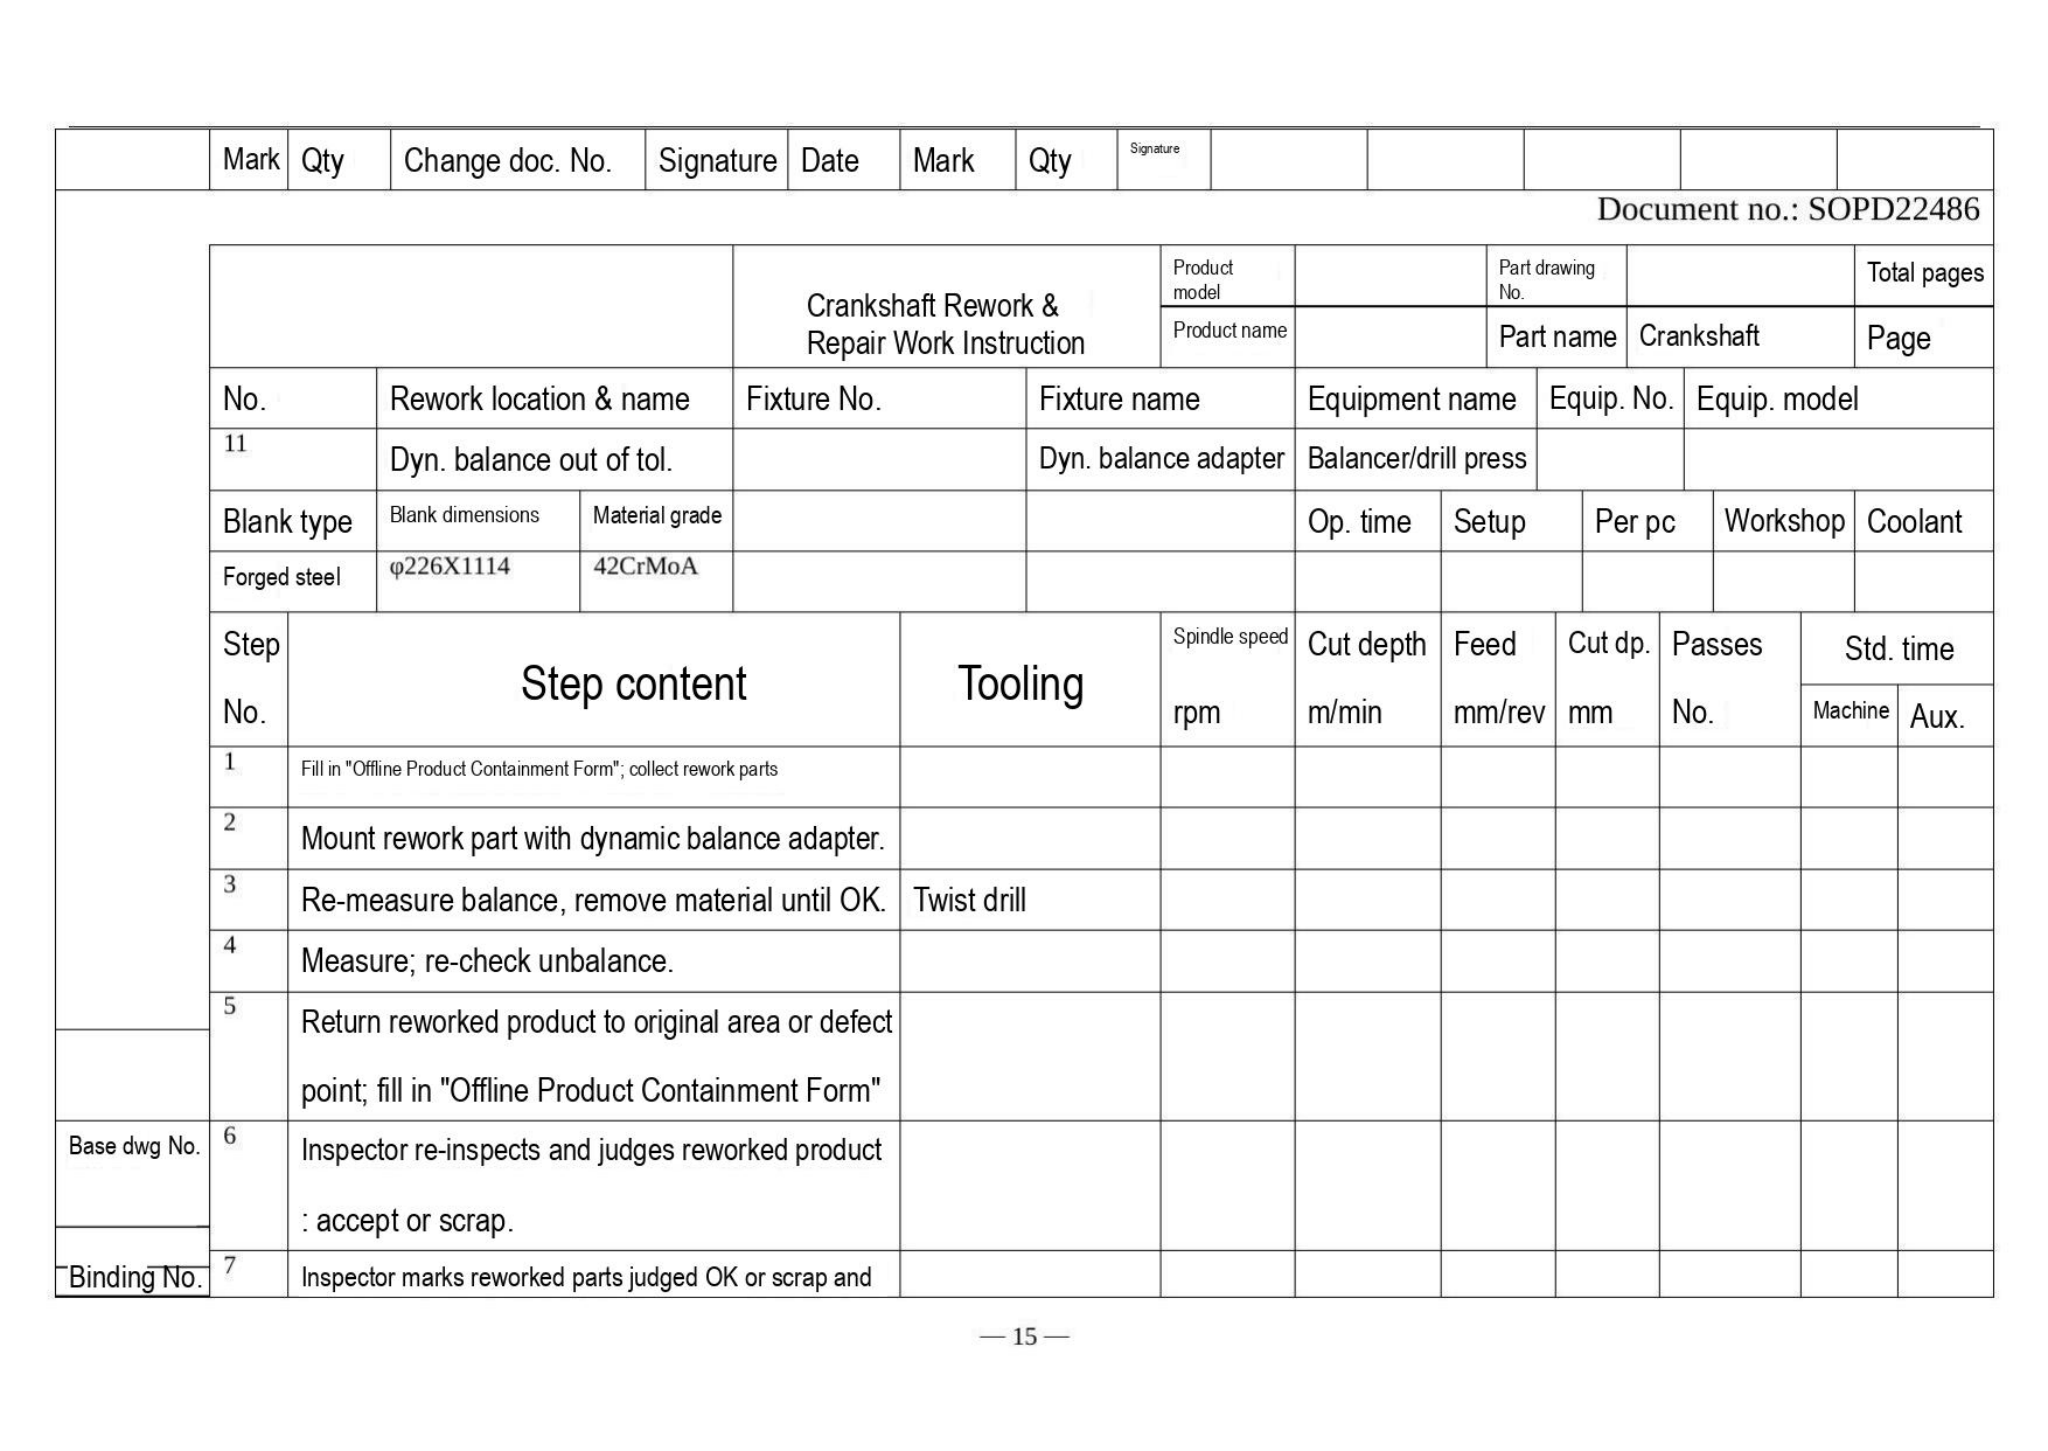| Mark | Qty | Change doc. No. | Signature | Date | Mark | Qty | Signature |
|---|---|---|---|---|---|---|---|

Document no.: SOPD22486

| | Crankshaft Rework & Repair Work Instruction | Product model | | Part drawing No. | | Total pages |
|---|---|---|---|---|---|---|
| | | Product name | | Part name | Crankshaft | Page |

| No. | Rework location & name | Fixture No. | Fixture name | Equipment name | Equip. No. | Equip. model |
|---|---|---|---|---|---|---|
| 11 | Dyn. balance out of tol. | | Dyn. balance adapter | Balancer/drill press | | |

| Blank type | Blank dimensions | Material grade | | | Op. time | Setup | Per pc | Workshop | Coolant |
|---|---|---|---|---|---|---|---|---|---|
| Forged steel | φ226X1114 | 42CrMoA | | | | | | | |

| Step No. | Step content | Tooling | Spindle speed rpm | Cut depth m/min | Feed mm/rev | Cut dp. mm | Passes No. | Std. time Machine | Std. time Aux. |
|---|---|---|---|---|---|---|---|---|---|
| 1 | Fill in "Offline Product Containment Form"; collect rework parts | | | | | | | | |
| 2 | Mount rework part with dynamic balance adapter. | | | | | | | | |
| 3 | Re-measure balance, remove material until OK. | Twist drill | | | | | | | |
| 4 | Measure; re-check unbalance. | | | | | | | | |
| 5 | Return reworked product to original area or defect point; fill in "Offline Product Containment Form" | | | | | | | | |
| 6 | Inspector re-inspects and judges reworked product : accept or scrap. | | | | | | | | |
| 7 | Inspector marks reworked parts judged OK or scrap and | | | | | | | | |

Base dwg No.

Binding No.

— 15 —
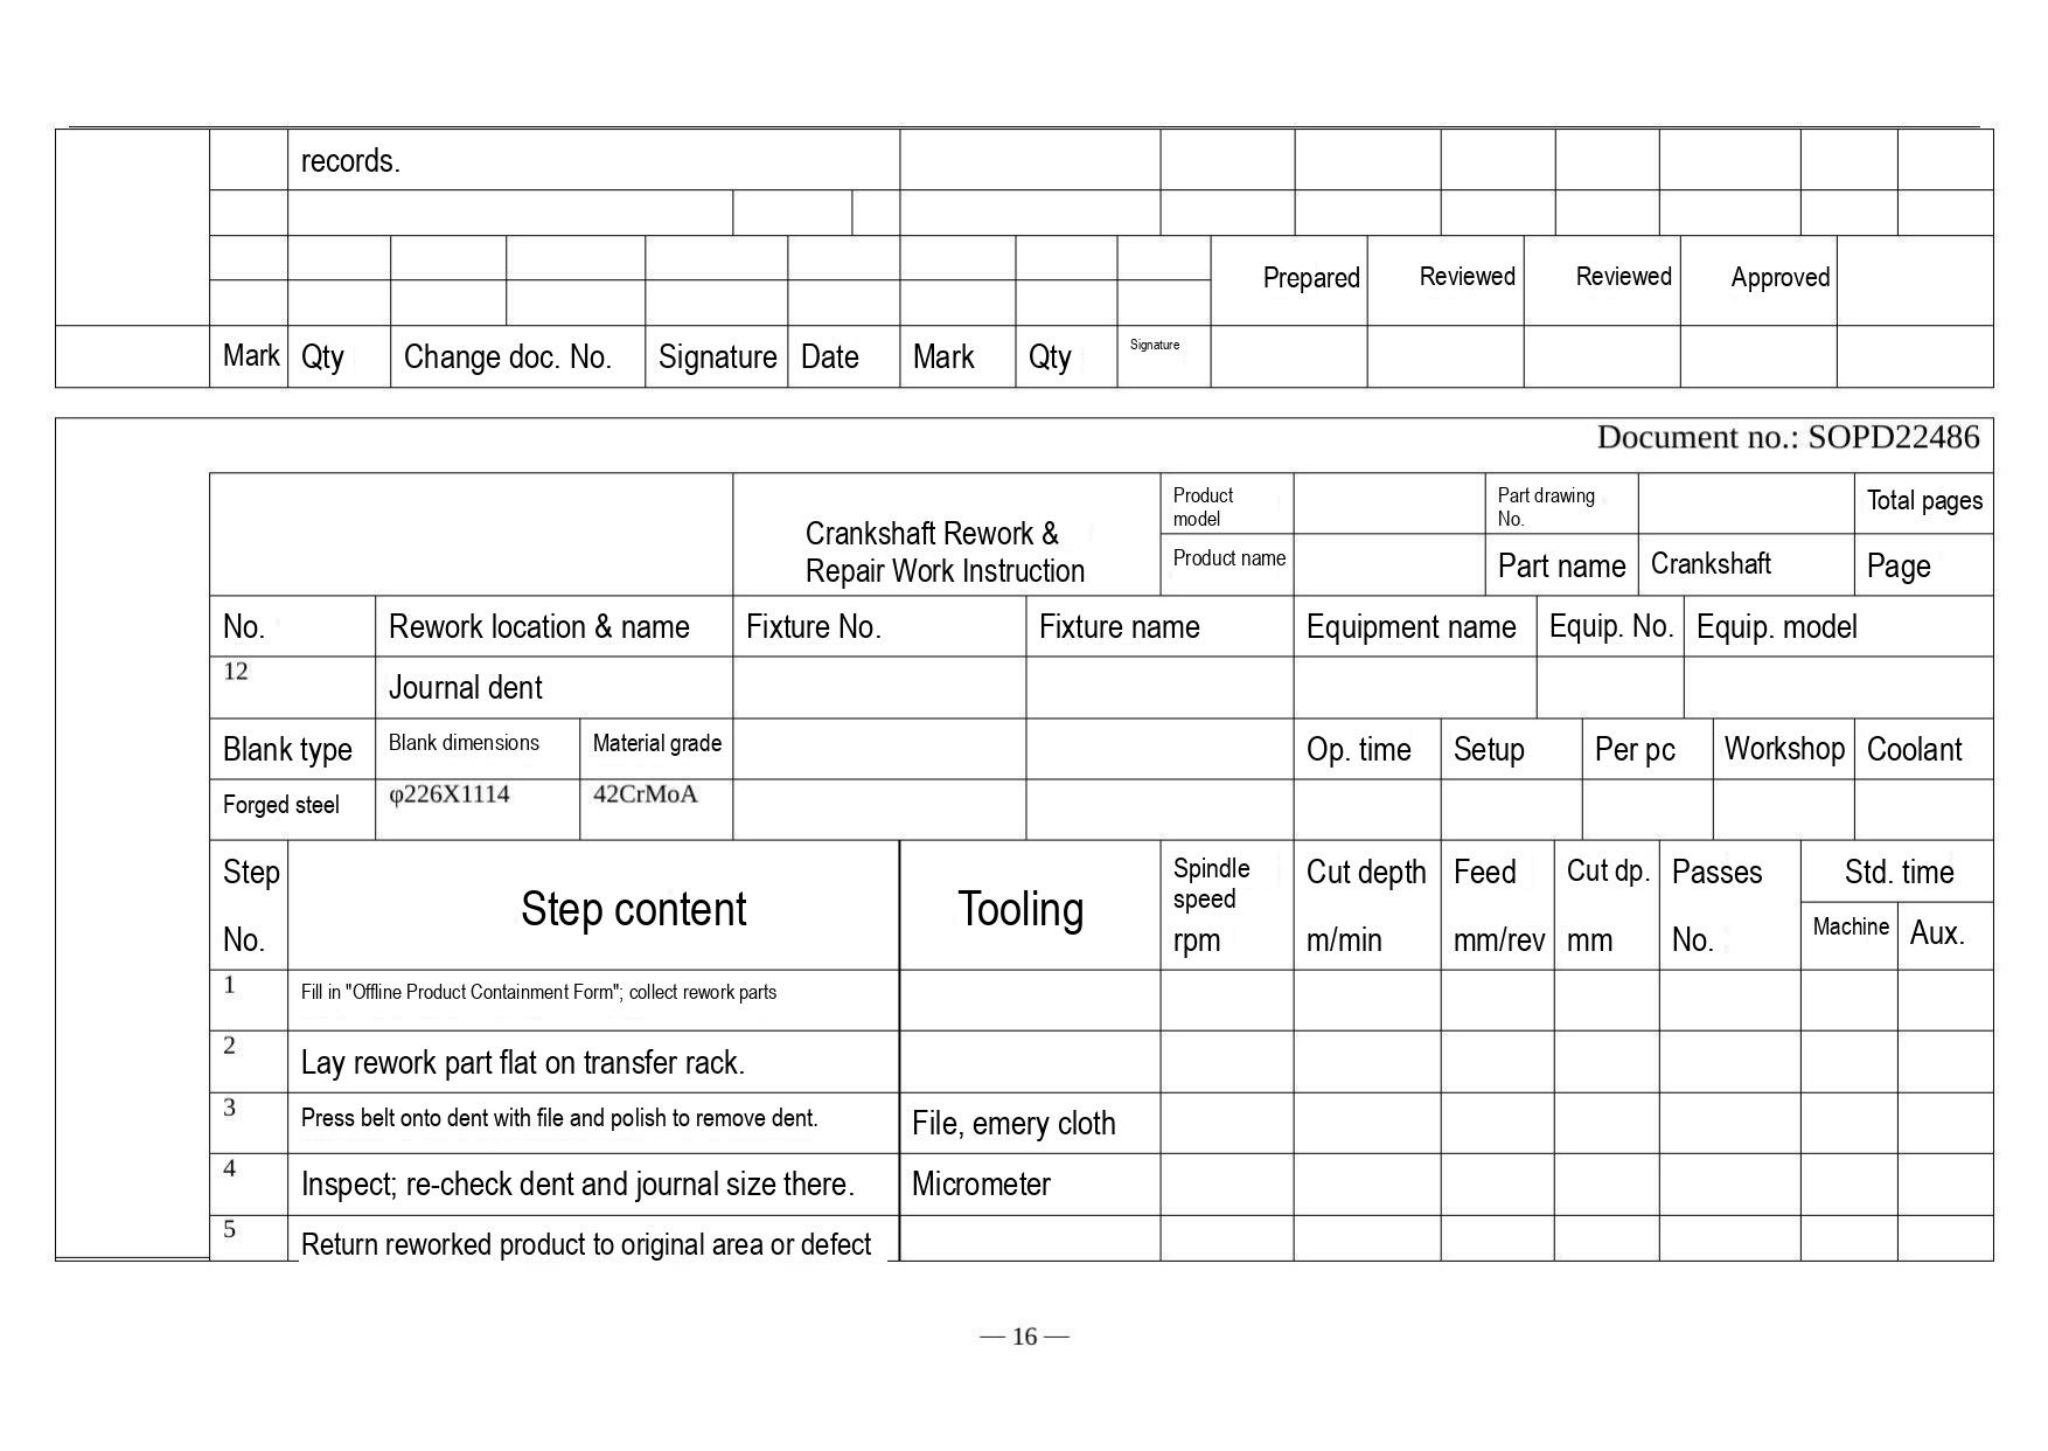| | | | | | | | | | | | | | |
|---|---|---|---|---|---|---|---|---|---|---|---|---|---|
| | records. | | | | | | | | | | | | |
| | | | | | | | | | | | | | |
| | | | | | | | | | Prepared | Reviewed | Reviewed | Approved | |
| Mark | Qty | Change doc. No. | Signature | Date | Mark | Qty | Signature | | | | | | |

Document no.: SOPD22486

| | Crankshaft Rework & Repair Work Instruction | Product model | | Part drawing No. | | Total pages |
|---|---|---|---|---|---|---|
| | | Product name | | Part name | Crankshaft | Page |

| No. | Rework location & name | Fixture No. | Fixture name | Equipment name | Equip. No. | Equip. model |
|---|---|---|---|---|---|---|
| 12 | Journal dent | | | | | |

| Blank type | Blank dimensions | Material grade | | | Op. time | Setup | Per pc | Workshop | Coolant |
|---|---|---|---|---|---|---|---|---|---|
| Forged steel | φ226X1114 | 42CrMoA | | | | | | | |

| Step No. | Step content | Tooling | Spindle speed rpm | Cut depth m/min | Feed mm/rev | Cut dp. mm | Passes No. | Std. time Machine | Std. time Aux. |
|---|---|---|---|---|---|---|---|---|---|
| 1 | Fill in "Offline Product Containment Form"; collect rework parts | | | | | | | | |
| 2 | Lay rework part flat on transfer rack. | | | | | | | | |
| 3 | Press belt onto dent with file and polish to remove dent. | File, emery cloth | | | | | | | |
| 4 | Inspect; re-check dent and journal size there. | Micrometer | | | | | | | |
| 5 | Return reworked product to original area or defect | | | | | | | | |

— 16 —
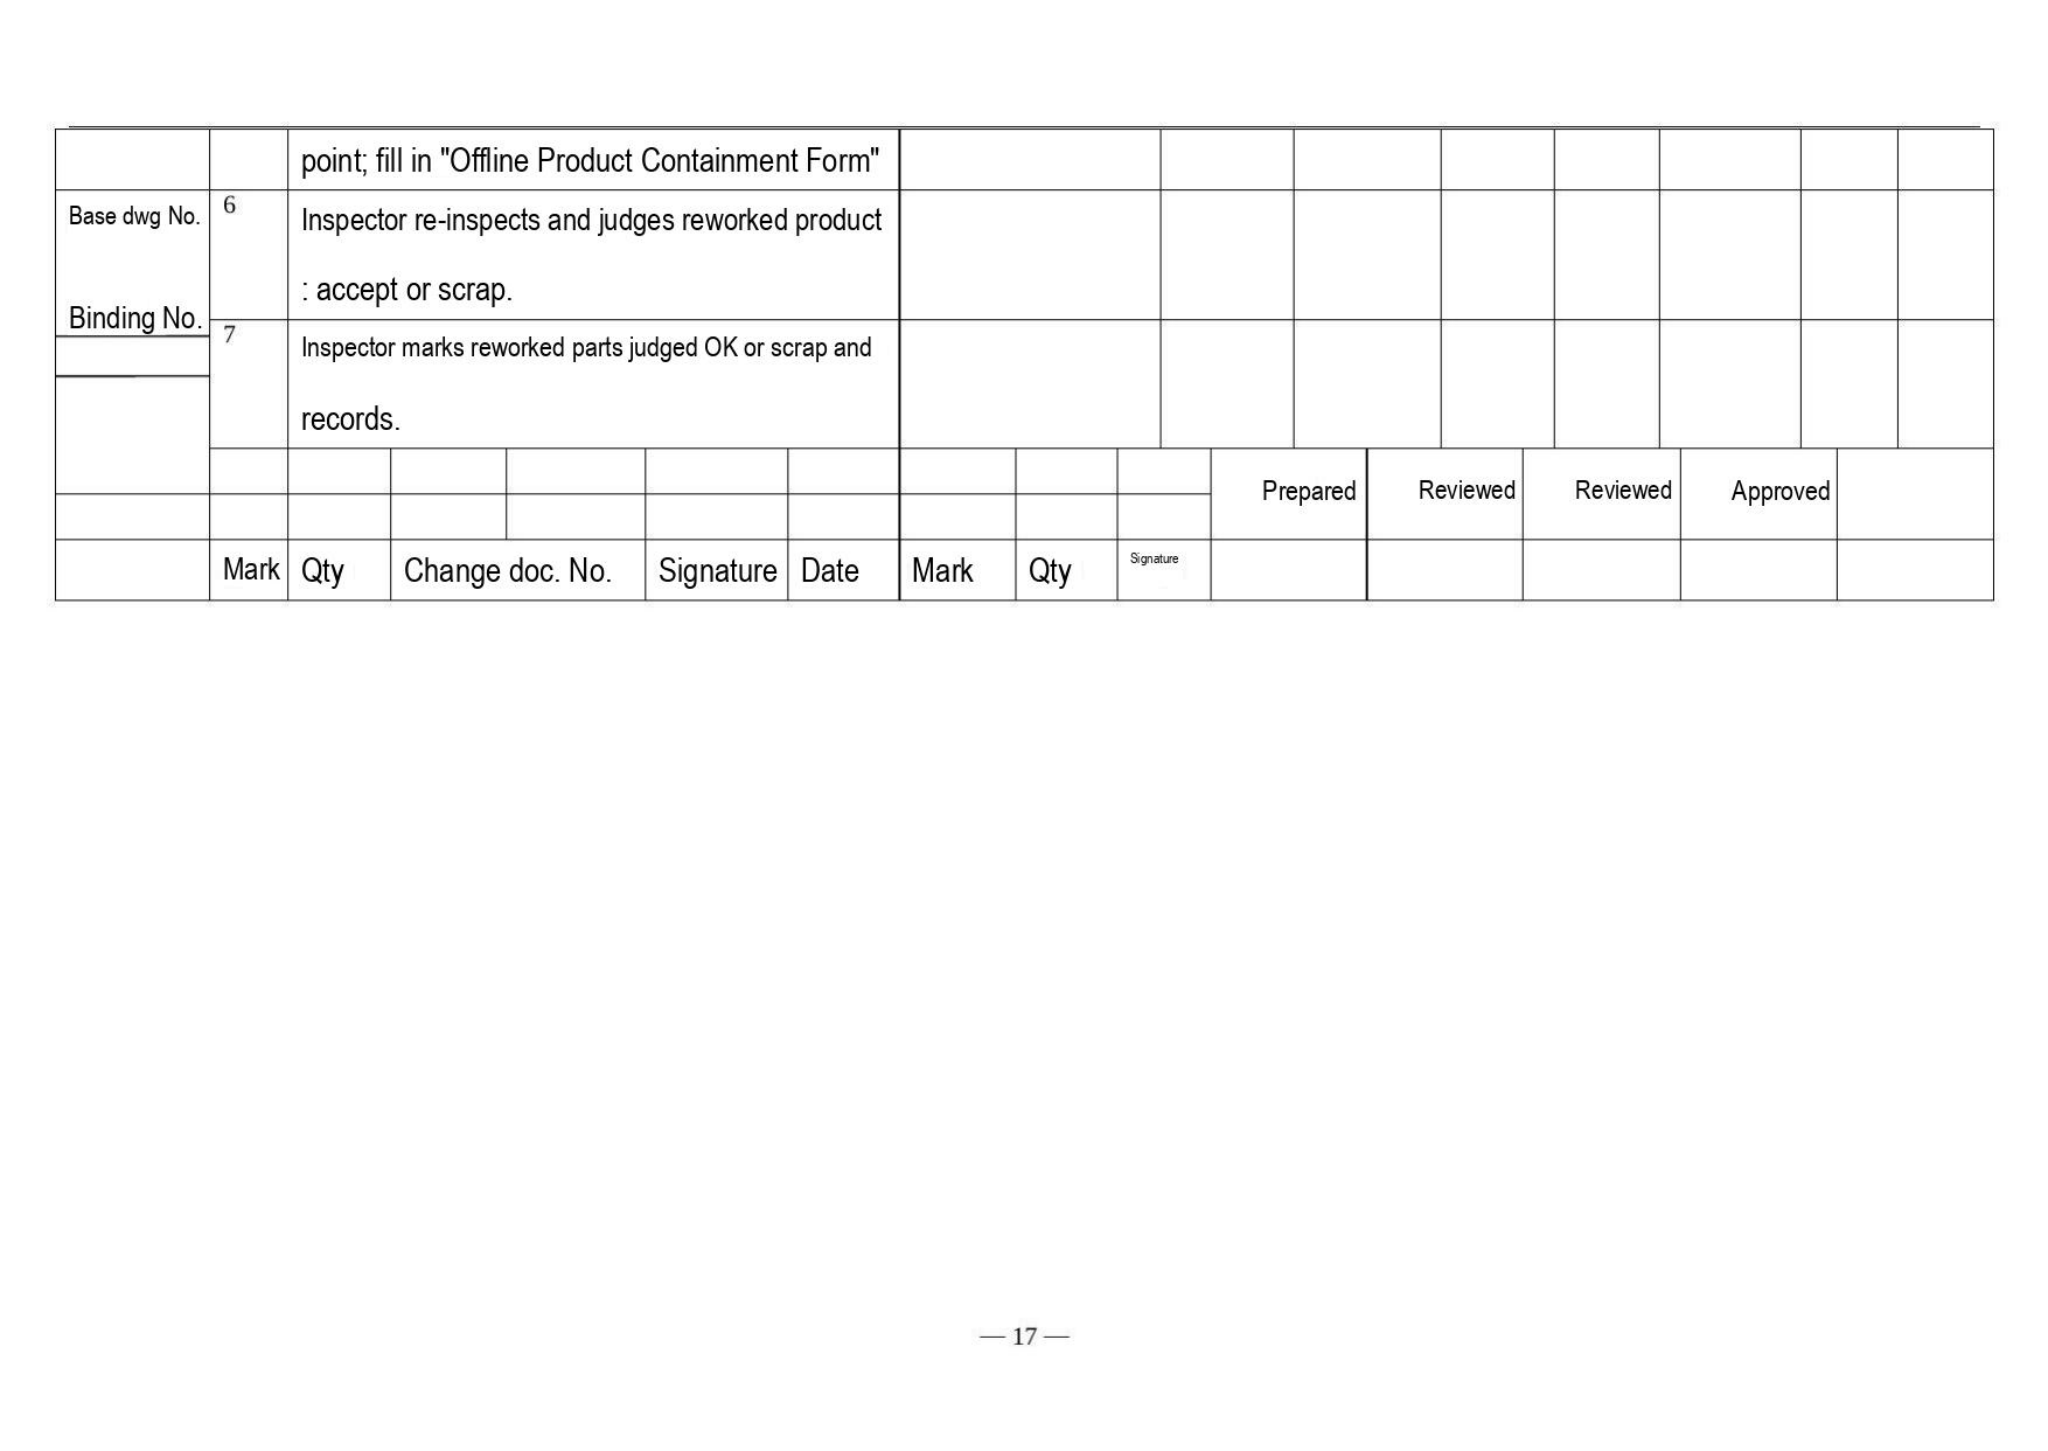| | | | | | | | | | |
|---|---|---|---|---|---|---|---|---|---|
| | | point; fill in "Offline Product Containment Form" | | | | | | | |
| Base dwg No. Binding No. | 6 | Inspector re-inspects and judges reworked product : accept or scrap. | | | | | | | |
| | 7 | Inspector marks reworked parts judged OK or scrap and records. | | | | | | | |

| | | | | | | | | | | | | | |
|---|---|---|---|---|---|---|---|---|---|---|---|---|---|
| | | | | | | | | | Prepared | Reviewed | Reviewed | Approved | |
| | | | | | | | | | | | | | |
| | Mark | Qty | Change doc. No. | Signature | Date | Mark | Qty | Signature | | | | | |

— 17 —